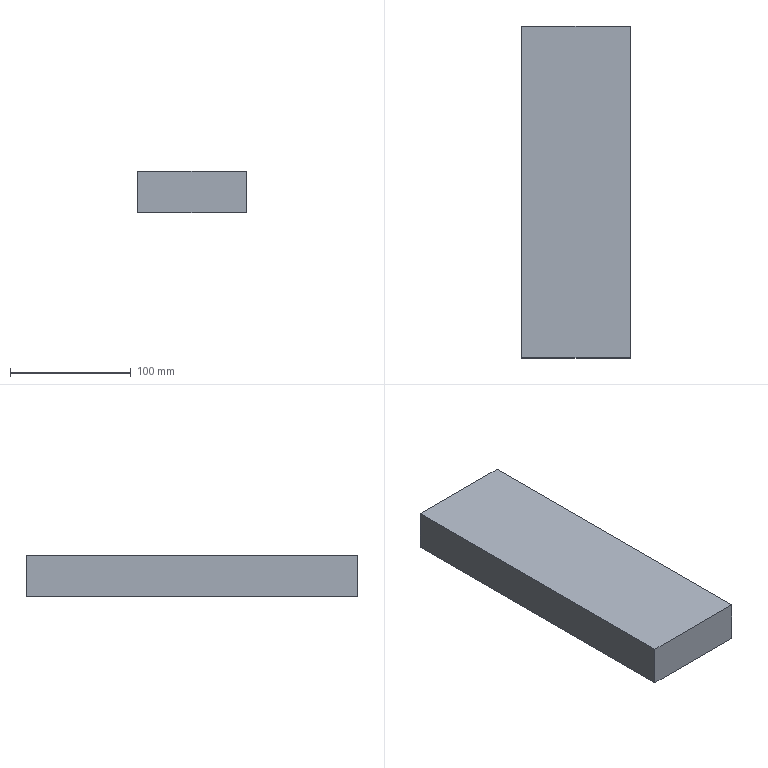Part | SolidWorks | features Extrusion 1 | 1 solid | 6 faces | box 90 x 275 x 34 mm | volume 841500 mm3 | plane 6
STEP:
#1=CARTESIAN_POINT('',(45.,-137.5,0.));
#2=VERTEX_POINT('',#1);
#3=CARTESIAN_POINT('',(45.,137.5,0.));
#4=VERTEX_POINT('',#3);
#5=CARTESIAN_POINT('',(45.,-137.5,0.));
#6=DIRECTION('',(0.,1.,0.));
#7=VECTOR('',#6,1000.);
#8=LINE('',#5,#7);
#9=EDGE_CURVE('',#2,#4,#8,.T.);
#10=ORIENTED_EDGE('',*,*,#9,.T.);
#11=CARTESIAN_POINT('',(45.,137.5,34.));
#12=VERTEX_POINT('',#11);
#13=CARTESIAN_POINT('',(45.,137.5,34.));
#14=DIRECTION('',(0.,0.,-1.));
#15=VECTOR('',#14,1000.);
#16=LINE('',#13,#15);
#17=EDGE_CURVE('',#12,#4,#16,.T.);
#18=ORIENTED_EDGE('',*,*,#17,.F.);
#19=CARTESIAN_POINT('',(45.,-137.5,34.));
#20=VERTEX_POINT('',#19);
#21=CARTESIAN_POINT('',(45.,-137.5,34.));
#22=DIRECTION('',(0.,1.,0.));
#23=VECTOR('',#22,1000.);
#24=LINE('',#21,#23);
#25=EDGE_CURVE('',#20,#12,#24,.T.);
#26=ORIENTED_EDGE('',*,*,#25,.F.);
#27=CARTESIAN_POINT('',(45.,-137.5,34.));
#28=DIRECTION('',(0.,0.,-1.));
#29=VECTOR('',#28,1000.);
#30=LINE('',#27,#29);
#31=EDGE_CURVE('',#20,#2,#30,.T.);
#32=ORIENTED_EDGE('',*,*,#31,.T.);
#33=EDGE_LOOP('',(#10,#18,#26,#32));
#34=FACE_OUTER_BOUND('',#33,.T.);
#35=CARTESIAN_POINT('',(45.,-137.5,34.));
#36=DIRECTION('',(-1.,0.,0.));
#37=DIRECTION('',(0.,0.,1.));
#38=AXIS2_PLACEMENT_3D('',#35,#36,#37);
#39=PLANE('',#38);
#40=ADVANCED_FACE('',(#34),#39,.F.);
#41=CARTESIAN_POINT('',(-45.,137.5,0.));
#42=VERTEX_POINT('',#41);
#43=CARTESIAN_POINT('',(-45.,137.5,0.));
#44=DIRECTION('',(-1.,0.,0.));
#45=VECTOR('',#44,1000.);
#46=LINE('',#43,#45);
#47=EDGE_CURVE('',#4,#42,#46,.T.);
#48=ORIENTED_EDGE('',*,*,#47,.T.);
#49=CARTESIAN_POINT('',(-45.,137.5,34.));
#50=VERTEX_POINT('',#49);
#51=CARTESIAN_POINT('',(-45.,137.5,34.));
#52=DIRECTION('',(0.,0.,-1.));
#53=VECTOR('',#52,1000.);
#54=LINE('',#51,#53);
#55=EDGE_CURVE('',#50,#42,#54,.T.);
#56=ORIENTED_EDGE('',*,*,#55,.F.);
#57=CARTESIAN_POINT('',(-45.,137.5,34.));
#58=DIRECTION('',(-1.,0.,0.));
#59=VECTOR('',#58,1000.);
#60=LINE('',#57,#59);
#61=EDGE_CURVE('',#12,#50,#60,.T.);
#62=ORIENTED_EDGE('',*,*,#61,.F.);
#63=ORIENTED_EDGE('',*,*,#17,.T.);
#64=EDGE_LOOP('',(#48,#56,#62,#63));
#65=FACE_OUTER_BOUND('',#64,.T.);
#66=CARTESIAN_POINT('',(-45.,137.5,34.));
#67=DIRECTION('',(0.,-1.,0.));
#68=DIRECTION('',(0.,0.,-1.));
#69=AXIS2_PLACEMENT_3D('',#66,#67,#68);
#70=PLANE('',#69);
#71=ADVANCED_FACE('',(#65),#70,.F.);
#72=CARTESIAN_POINT('',(-45.,-137.5,0.));
#73=VERTEX_POINT('',#72);
#74=CARTESIAN_POINT('',(-45.,-137.5,0.));
#75=DIRECTION('',(0.,-1.,0.));
#76=VECTOR('',#75,1000.);
#77=LINE('',#74,#76);
#78=EDGE_CURVE('',#42,#73,#77,.T.);
#79=ORIENTED_EDGE('',*,*,#78,.T.);
#80=CARTESIAN_POINT('',(-45.,-137.5,34.));
#81=VERTEX_POINT('',#80);
#82=CARTESIAN_POINT('',(-45.,-137.5,34.));
#83=DIRECTION('',(0.,0.,-1.));
#84=VECTOR('',#83,1000.);
#85=LINE('',#82,#84);
#86=EDGE_CURVE('',#81,#73,#85,.T.);
#87=ORIENTED_EDGE('',*,*,#86,.F.);
#88=CARTESIAN_POINT('',(-45.,-137.5,34.));
#89=DIRECTION('',(0.,-1.,0.));
#90=VECTOR('',#89,1000.);
#91=LINE('',#88,#90);
#92=EDGE_CURVE('',#50,#81,#91,.T.);
#93=ORIENTED_EDGE('',*,*,#92,.F.);
#94=ORIENTED_EDGE('',*,*,#55,.T.);
#95=EDGE_LOOP('',(#79,#87,#93,#94));
#96=FACE_OUTER_BOUND('',#95,.T.);
#97=CARTESIAN_POINT('',(-45.,-137.5,34.));
#98=DIRECTION('',(1.,0.,0.));
#99=DIRECTION('',(0.,0.,-1.));
#100=AXIS2_PLACEMENT_3D('',#97,#98,#99);
#101=PLANE('',#100);
#102=ADVANCED_FACE('',(#96),#101,.F.);
#103=CARTESIAN_POINT('',(-45.,-137.5,0.));
#104=DIRECTION('',(1.,0.,0.));
#105=VECTOR('',#104,1000.);
#106=LINE('',#103,#105);
#107=EDGE_CURVE('',#73,#2,#106,.T.);
#108=ORIENTED_EDGE('',*,*,#107,.T.);
#109=ORIENTED_EDGE('',*,*,#31,.F.);
#110=CARTESIAN_POINT('',(-45.,-137.5,34.));
#111=DIRECTION('',(1.,0.,0.));
#112=VECTOR('',#111,1000.);
#113=LINE('',#110,#112);
#114=EDGE_CURVE('',#81,#20,#113,.T.);
#115=ORIENTED_EDGE('',*,*,#114,.F.);
#116=ORIENTED_EDGE('',*,*,#86,.T.);
#117=EDGE_LOOP('',(#108,#109,#115,#116));
#118=FACE_OUTER_BOUND('',#117,.T.);
#119=CARTESIAN_POINT('',(-45.,-137.5,34.));
#120=DIRECTION('',(0.,1.,0.));
#121=DIRECTION('',(0.,0.,1.));
#122=AXIS2_PLACEMENT_3D('',#119,#120,#121);
#123=PLANE('',#122);
#124=ADVANCED_FACE('',(#118),#123,.F.);
#125=ORIENTED_EDGE('',*,*,#25,.T.);
#126=ORIENTED_EDGE('',*,*,#61,.T.);
#127=ORIENTED_EDGE('',*,*,#92,.T.);
#128=ORIENTED_EDGE('',*,*,#114,.T.);
#129=EDGE_LOOP('',(#125,#126,#127,#128));
#130=FACE_OUTER_BOUND('',#129,.T.);
#131=CARTESIAN_POINT('',(0.,0.,34.));
#132=DIRECTION('',(0.,0.,-1.));
#133=DIRECTION('',(-1.,0.,0.));
#134=AXIS2_PLACEMENT_3D('',#131,#132,#133);
#135=PLANE('',#134);
#136=ADVANCED_FACE('',(#130),#135,.F.);
#137=ORIENTED_EDGE('',*,*,#9,.F.);
#138=ORIENTED_EDGE('',*,*,#107,.F.);
#139=ORIENTED_EDGE('',*,*,#78,.F.);
#140=ORIENTED_EDGE('',*,*,#47,.F.);
#141=EDGE_LOOP('',(#137,#138,#139,#140));
#142=FACE_OUTER_BOUND('',#141,.T.);
#143=CARTESIAN_POINT('',(0.,0.,0.));
#144=DIRECTION('',(0.,0.,-1.));
#145=DIRECTION('',(-1.,0.,0.));
#146=AXIS2_PLACEMENT_3D('',#143,#144,#145);
#147=PLANE('',#146);
#148=ADVANCED_FACE('',(#142),#147,.T.);
#149=CLOSED_SHELL('',(#40,#71,#102,#124,#136,#148));
#150=MANIFOLD_SOLID_BREP('',#149);
#151=CARTESIAN_POINT('',(0.,0.,0.));
#152=DIRECTION('',(0.,0.,1.));
#153=DIRECTION('',(1.,0.,0.));
#154=AXIS2_PLACEMENT_3D('',#151,#152,#153);
#155=(LENGTH_UNIT()NAMED_UNIT(*)SI_UNIT(.MILLI.,.METRE.));
#156=UNCERTAINTY_MEASURE_WITH_UNIT(LENGTH_MEASURE(0.00001),#155,'','');
#157=(NAMED_UNIT(*)PLANE_ANGLE_UNIT()SI_UNIT($,.RADIAN.));
#158=(NAMED_UNIT(*)SI_UNIT($,.STERADIAN.)SOLID_ANGLE_UNIT());
#159=(GEOMETRIC_REPRESENTATION_CONTEXT(3)GLOBAL_UNCERTAINTY_ASSIGNED_CONTEXT((#156))GLOBAL_UNIT_ASSIGNED_CONTEXT((#155,#157,#158))REPRESENTATION_CONTEXT('',''));
#160=ADVANCED_BREP_SHAPE_REPRESENTATION('',(#150,#154),#159);